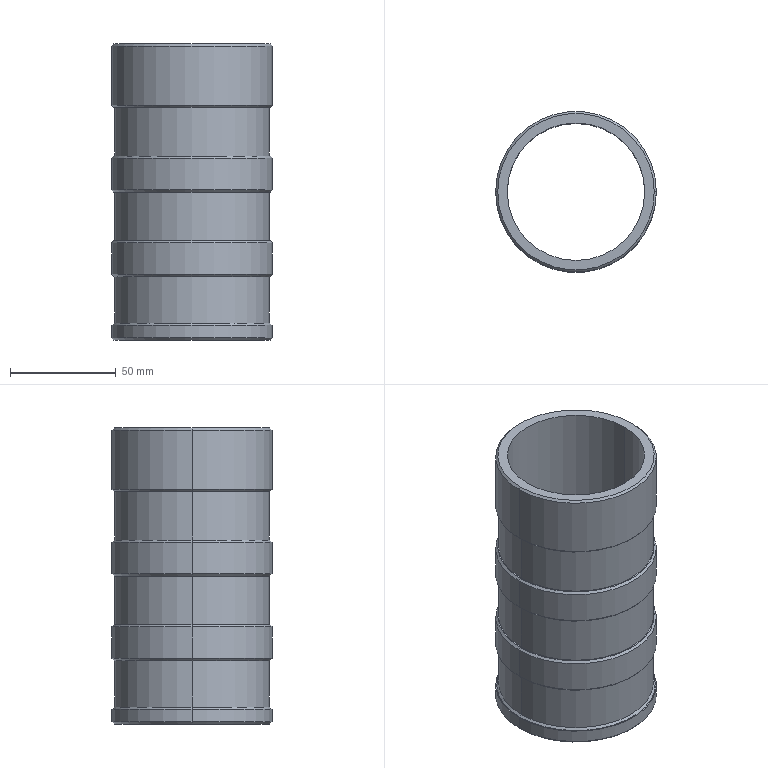Part | SolidWorks | features Chamfer 2, Extrusion 1, ICE 1, LPattern 1 | 1 solid | 40 faces | box 76 x 76 x 140 mm | volume 145605 mm3 | cone 16 | cylinder 16 | plane 8 | commonest cylinder face diameters 76 x8 73 x6 65 x2
STEP:
#1=CARTESIAN_POINT('',(-37.,0.,110.));
#2=VERTEX_POINT('',#1);
#3=CARTESIAN_POINT('',(37.,0.,110.));
#4=VERTEX_POINT('',#3);
#5=CARTESIAN_POINT('',(0.,0.,110.));
#6=DIRECTION('',(0.,0.,-1.));
#7=DIRECTION('',(1.,0.,0.));
#8=AXIS2_PLACEMENT_3D('',#5,#6,#7);
#9=CIRCLE('',#8,37.);
#10=EDGE_CURVE('',#2,#4,#9,.T.);
#11=ORIENTED_EDGE('',*,*,#10,.F.);
#12=CARTESIAN_POINT('',(-38.,0.,111.));
#13=VERTEX_POINT('',#12);
#14=CARTESIAN_POINT('',(-38.,0.,111.));
#15=DIRECTION('',(-0.7071,0.,0.7071));
#16=VECTOR('',#15,1000.);
#17=LINE('',#14,#16);
#18=EDGE_CURVE('',#2,#13,#17,.T.);
#19=ORIENTED_EDGE('',*,*,#18,.T.);
#20=CARTESIAN_POINT('',(38.,0.,111.));
#21=VERTEX_POINT('',#20);
#22=CARTESIAN_POINT('',(0.,0.,111.));
#23=DIRECTION('',(0.,0.,1.));
#24=DIRECTION('',(1.,0.,0.));
#25=AXIS2_PLACEMENT_3D('',#22,#23,#24);
#26=CIRCLE('',#25,38.);
#27=EDGE_CURVE('',#21,#13,#26,.T.);
#28=ORIENTED_EDGE('',*,*,#27,.F.);
#29=CARTESIAN_POINT('',(38.,0.,111.));
#30=DIRECTION('',(0.7071,0.,0.7071));
#31=VECTOR('',#30,1000.);
#32=LINE('',#29,#31);
#33=EDGE_CURVE('',#4,#21,#32,.T.);
#34=ORIENTED_EDGE('',*,*,#33,.F.);
#35=EDGE_LOOP('',(#11,#19,#28,#34));
#36=FACE_OUTER_BOUND('',#35,.T.);
#37=CARTESIAN_POINT('',(0.,0.,111.));
#38=DIRECTION('',(0.,0.,1.));
#39=DIRECTION('',(1.,0.,0.));
#40=AXIS2_PLACEMENT_3D('',#37,#38,#39);
#41=CONICAL_SURFACE('',#40,38.,0.7854);
#42=ADVANCED_FACE('',(#36),#41,.T.);
#43=CARTESIAN_POINT('',(37.,0.,87.));
#44=VERTEX_POINT('',#43);
#45=CARTESIAN_POINT('',(-37.,0.,87.));
#46=VERTEX_POINT('',#45);
#47=CARTESIAN_POINT('',(0.,0.,87.));
#48=DIRECTION('',(0.,0.,1.));
#49=DIRECTION('',(1.,0.,0.));
#50=AXIS2_PLACEMENT_3D('',#47,#48,#49);
#51=CIRCLE('',#50,37.);
#52=EDGE_CURVE('',#44,#46,#51,.T.);
#53=ORIENTED_EDGE('',*,*,#52,.F.);
#54=CARTESIAN_POINT('',(38.,0.,86.));
#55=VERTEX_POINT('',#54);
#56=CARTESIAN_POINT('',(37.,0.,87.));
#57=DIRECTION('',(0.7071,0.,-0.7071));
#58=VECTOR('',#57,1000.);
#59=LINE('',#56,#58);
#60=EDGE_CURVE('',#44,#55,#59,.T.);
#61=ORIENTED_EDGE('',*,*,#60,.T.);
#62=CARTESIAN_POINT('',(-38.,0.,86.));
#63=VERTEX_POINT('',#62);
#64=CARTESIAN_POINT('',(0.,0.,86.));
#65=DIRECTION('',(0.,0.,-1.));
#66=DIRECTION('',(1.,0.,0.));
#67=AXIS2_PLACEMENT_3D('',#64,#65,#66);
#68=CIRCLE('',#67,38.);
#69=EDGE_CURVE('',#63,#55,#68,.T.);
#70=ORIENTED_EDGE('',*,*,#69,.F.);
#71=CARTESIAN_POINT('',(-37.,0.,87.));
#72=DIRECTION('',(-0.7071,0.,-0.7071));
#73=VECTOR('',#72,1000.);
#74=LINE('',#71,#73);
#75=EDGE_CURVE('',#46,#63,#74,.T.);
#76=ORIENTED_EDGE('',*,*,#75,.F.);
#77=EDGE_LOOP('',(#53,#61,#70,#76));
#78=FACE_OUTER_BOUND('',#77,.T.);
#79=CARTESIAN_POINT('',(0.,0.,87.));
#80=DIRECTION('',(0.,0.,-1.));
#81=DIRECTION('',(-1.,0.,0.));
#82=AXIS2_PLACEMENT_3D('',#79,#80,#81);
#83=CONICAL_SURFACE('',#82,37.,0.7854);
#84=ADVANCED_FACE('',(#78),#83,.T.);
#85=CARTESIAN_POINT('',(-37.,0.,70.));
#86=VERTEX_POINT('',#85);
#87=CARTESIAN_POINT('',(37.,0.,70.));
#88=VERTEX_POINT('',#87);
#89=CARTESIAN_POINT('',(0.,0.,70.));
#90=DIRECTION('',(0.,0.,-1.));
#91=DIRECTION('',(1.,0.,0.));
#92=AXIS2_PLACEMENT_3D('',#89,#90,#91);
#93=CIRCLE('',#92,37.);
#94=EDGE_CURVE('',#86,#88,#93,.T.);
#95=ORIENTED_EDGE('',*,*,#94,.F.);
#96=CARTESIAN_POINT('',(-38.,0.,71.));
#97=VERTEX_POINT('',#96);
#98=CARTESIAN_POINT('',(-38.,0.,71.));
#99=DIRECTION('',(-0.7071,0.,0.7071));
#100=VECTOR('',#99,1000.);
#101=LINE('',#98,#100);
#102=EDGE_CURVE('',#86,#97,#101,.T.);
#103=ORIENTED_EDGE('',*,*,#102,.T.);
#104=CARTESIAN_POINT('',(38.,0.,71.));
#105=VERTEX_POINT('',#104);
#106=CARTESIAN_POINT('',(0.,0.,71.));
#107=DIRECTION('',(0.,0.,1.));
#108=DIRECTION('',(1.,0.,0.));
#109=AXIS2_PLACEMENT_3D('',#106,#107,#108);
#110=CIRCLE('',#109,38.);
#111=EDGE_CURVE('',#105,#97,#110,.T.);
#112=ORIENTED_EDGE('',*,*,#111,.F.);
#113=CARTESIAN_POINT('',(38.,0.,71.));
#114=DIRECTION('',(0.7071,0.,0.7071));
#115=VECTOR('',#114,1000.);
#116=LINE('',#113,#115);
#117=EDGE_CURVE('',#88,#105,#116,.T.);
#118=ORIENTED_EDGE('',*,*,#117,.F.);
#119=EDGE_LOOP('',(#95,#103,#112,#118));
#120=FACE_OUTER_BOUND('',#119,.T.);
#121=CARTESIAN_POINT('',(0.,0.,71.));
#122=DIRECTION('',(0.,0.,1.));
#123=DIRECTION('',(1.,0.,0.));
#124=AXIS2_PLACEMENT_3D('',#121,#122,#123);
#125=CONICAL_SURFACE('',#124,38.,0.7854);
#126=ADVANCED_FACE('',(#120),#125,.T.);
#127=CARTESIAN_POINT('',(37.,0.,47.));
#128=VERTEX_POINT('',#127);
#129=CARTESIAN_POINT('',(-37.,0.,47.));
#130=VERTEX_POINT('',#129);
#131=CARTESIAN_POINT('',(0.,0.,47.));
#132=DIRECTION('',(0.,0.,1.));
#133=DIRECTION('',(1.,0.,0.));
#134=AXIS2_PLACEMENT_3D('',#131,#132,#133);
#135=CIRCLE('',#134,37.);
#136=EDGE_CURVE('',#128,#130,#135,.T.);
#137=ORIENTED_EDGE('',*,*,#136,.F.);
#138=CARTESIAN_POINT('',(38.,0.,46.));
#139=VERTEX_POINT('',#138);
#140=CARTESIAN_POINT('',(37.,0.,47.));
#141=DIRECTION('',(0.7071,0.,-0.7071));
#142=VECTOR('',#141,1000.);
#143=LINE('',#140,#142);
#144=EDGE_CURVE('',#128,#139,#143,.T.);
#145=ORIENTED_EDGE('',*,*,#144,.T.);
#146=CARTESIAN_POINT('',(-38.,0.,46.));
#147=VERTEX_POINT('',#146);
#148=CARTESIAN_POINT('',(0.,0.,46.));
#149=DIRECTION('',(0.,0.,-1.));
#150=DIRECTION('',(1.,0.,0.));
#151=AXIS2_PLACEMENT_3D('',#148,#149,#150);
#152=CIRCLE('',#151,38.);
#153=EDGE_CURVE('',#147,#139,#152,.T.);
#154=ORIENTED_EDGE('',*,*,#153,.F.);
#155=CARTESIAN_POINT('',(-37.,0.,47.));
#156=DIRECTION('',(-0.7071,0.,-0.7071));
#157=VECTOR('',#156,1000.);
#158=LINE('',#155,#157);
#159=EDGE_CURVE('',#130,#147,#158,.T.);
#160=ORIENTED_EDGE('',*,*,#159,.F.);
#161=EDGE_LOOP('',(#137,#145,#154,#160));
#162=FACE_OUTER_BOUND('',#161,.T.);
#163=CARTESIAN_POINT('',(0.,0.,47.));
#164=DIRECTION('',(0.,0.,-1.));
#165=DIRECTION('',(-1.,0.,0.));
#166=AXIS2_PLACEMENT_3D('',#163,#164,#165);
#167=CONICAL_SURFACE('',#166,37.,0.7854);
#168=ADVANCED_FACE('',(#162),#167,.T.);
#169=CARTESIAN_POINT('',(-37.,0.,30.));
#170=VERTEX_POINT('',#169);
#171=CARTESIAN_POINT('',(37.,0.,30.));
#172=VERTEX_POINT('',#171);
#173=CARTESIAN_POINT('',(0.,0.,30.));
#174=DIRECTION('',(0.,0.,-1.));
#175=DIRECTION('',(1.,0.,0.));
#176=AXIS2_PLACEMENT_3D('',#173,#174,#175);
#177=CIRCLE('',#176,37.);
#178=EDGE_CURVE('',#170,#172,#177,.T.);
#179=ORIENTED_EDGE('',*,*,#178,.F.);
#180=CARTESIAN_POINT('',(-38.,0.,31.));
#181=VERTEX_POINT('',#180);
#182=CARTESIAN_POINT('',(-38.,0.,31.));
#183=DIRECTION('',(-0.7071,0.,0.7071));
#184=VECTOR('',#183,1000.);
#185=LINE('',#182,#184);
#186=EDGE_CURVE('',#170,#181,#185,.T.);
#187=ORIENTED_EDGE('',*,*,#186,.T.);
#188=CARTESIAN_POINT('',(38.,0.,31.));
#189=VERTEX_POINT('',#188);
#190=CARTESIAN_POINT('',(0.,0.,31.));
#191=DIRECTION('',(0.,0.,1.));
#192=DIRECTION('',(1.,0.,0.));
#193=AXIS2_PLACEMENT_3D('',#190,#191,#192);
#194=CIRCLE('',#193,38.);
#195=EDGE_CURVE('',#189,#181,#194,.T.);
#196=ORIENTED_EDGE('',*,*,#195,.F.);
#197=CARTESIAN_POINT('',(38.,0.,31.));
#198=DIRECTION('',(0.7071,0.,0.7071));
#199=VECTOR('',#198,1000.);
#200=LINE('',#197,#199);
#201=EDGE_CURVE('',#172,#189,#200,.T.);
#202=ORIENTED_EDGE('',*,*,#201,.F.);
#203=EDGE_LOOP('',(#179,#187,#196,#202));
#204=FACE_OUTER_BOUND('',#203,.T.);
#205=CARTESIAN_POINT('',(0.,0.,31.));
#206=DIRECTION('',(0.,0.,1.));
#207=DIRECTION('',(1.,0.,0.));
#208=AXIS2_PLACEMENT_3D('',#205,#206,#207);
#209=CONICAL_SURFACE('',#208,38.,0.7854);
#210=ADVANCED_FACE('',(#204),#209,.T.);
#211=CARTESIAN_POINT('',(36.5,0.,8.));
#212=VERTEX_POINT('',#211);
#213=CARTESIAN_POINT('',(-36.5,0.,8.));
#214=VERTEX_POINT('',#213);
#215=CARTESIAN_POINT('',(0.,0.,8.));
#216=DIRECTION('',(0.,0.,1.));
#217=DIRECTION('',(1.,0.,0.));
#218=AXIS2_PLACEMENT_3D('',#215,#216,#217);
#219=CIRCLE('',#218,36.5);
#220=EDGE_CURVE('',#212,#214,#219,.T.);
#221=ORIENTED_EDGE('',*,*,#220,.F.);
#222=CARTESIAN_POINT('',(37.5,0.,7.));
#223=VERTEX_POINT('',#222);
#224=CARTESIAN_POINT('',(36.5,0.,8.));
#225=DIRECTION('',(0.7071,0.,-0.7071));
#226=VECTOR('',#225,1000.);
#227=LINE('',#224,#226);
#228=EDGE_CURVE('',#212,#223,#227,.T.);
#229=ORIENTED_EDGE('',*,*,#228,.T.);
#230=CARTESIAN_POINT('',(-37.5,0.,7.));
#231=VERTEX_POINT('',#230);
#232=CARTESIAN_POINT('',(0.,0.,7.));
#233=DIRECTION('',(0.,0.,-1.));
#234=DIRECTION('',(1.,0.,0.));
#235=AXIS2_PLACEMENT_3D('',#232,#233,#234);
#236=CIRCLE('',#235,37.5);
#237=EDGE_CURVE('',#231,#223,#236,.T.);
#238=ORIENTED_EDGE('',*,*,#237,.F.);
#239=CARTESIAN_POINT('',(-36.5,0.,8.));
#240=DIRECTION('',(-0.7071,0.,-0.7071));
#241=VECTOR('',#240,1000.);
#242=LINE('',#239,#241);
#243=EDGE_CURVE('',#214,#231,#242,.T.);
#244=ORIENTED_EDGE('',*,*,#243,.F.);
#245=EDGE_LOOP('',(#221,#229,#238,#244));
#246=FACE_OUTER_BOUND('',#245,.T.);
#247=CARTESIAN_POINT('',(0.,0.,8.));
#248=DIRECTION('',(0.,0.,-1.));
#249=DIRECTION('',(-1.,0.,0.));
#250=AXIS2_PLACEMENT_3D('',#247,#248,#249);
#251=CONICAL_SURFACE('',#250,36.5,0.7854);
#252=ADVANCED_FACE('',(#246),#251,.T.);
#253=CARTESIAN_POINT('',(-37.,0.,0.));
#254=VERTEX_POINT('',#253);
#255=CARTESIAN_POINT('',(37.,0.,0.));
#256=VERTEX_POINT('',#255);
#257=CARTESIAN_POINT('',(0.,0.,0.));
#258=DIRECTION('',(0.,0.,-1.));
#259=DIRECTION('',(1.,0.,0.));
#260=AXIS2_PLACEMENT_3D('',#257,#258,#259);
#261=CIRCLE('',#260,37.);
#262=EDGE_CURVE('',#254,#256,#261,.T.);
#263=ORIENTED_EDGE('',*,*,#262,.F.);
#264=CARTESIAN_POINT('',(-38.,0.,1.));
#265=VERTEX_POINT('',#264);
#266=CARTESIAN_POINT('',(-38.,0.,1.));
#267=DIRECTION('',(-0.7071,0.,0.7071));
#268=VECTOR('',#267,1000.);
#269=LINE('',#266,#268);
#270=EDGE_CURVE('',#254,#265,#269,.T.);
#271=ORIENTED_EDGE('',*,*,#270,.T.);
#272=CARTESIAN_POINT('',(38.,0.,1.));
#273=VERTEX_POINT('',#272);
#274=CARTESIAN_POINT('',(0.,0.,1.));
#275=DIRECTION('',(0.,0.,1.));
#276=DIRECTION('',(1.,0.,0.));
#277=AXIS2_PLACEMENT_3D('',#274,#275,#276);
#278=CIRCLE('',#277,38.);
#279=EDGE_CURVE('',#273,#265,#278,.T.);
#280=ORIENTED_EDGE('',*,*,#279,.F.);
#281=CARTESIAN_POINT('',(38.,0.,1.));
#282=DIRECTION('',(0.7071,0.,0.7071));
#283=VECTOR('',#282,1000.);
#284=LINE('',#281,#283);
#285=EDGE_CURVE('',#256,#273,#284,.T.);
#286=ORIENTED_EDGE('',*,*,#285,.F.);
#287=EDGE_LOOP('',(#263,#271,#280,#286));
#288=FACE_OUTER_BOUND('',#287,.T.);
#289=CARTESIAN_POINT('',(0.,0.,1.));
#290=DIRECTION('',(0.,0.,1.));
#291=DIRECTION('',(1.,0.,0.));
#292=AXIS2_PLACEMENT_3D('',#289,#290,#291);
#293=CONICAL_SURFACE('',#292,38.,0.7854);
#294=ADVANCED_FACE('',(#288),#293,.T.);
#295=ORIENTED_EDGE('',*,*,#153,.T.);
#296=CARTESIAN_POINT('',(38.,0.,140.));
#297=DIRECTION('',(0.,0.,-1.));
#298=VECTOR('',#297,1000.);
#299=LINE('',#296,#298);
#300=EDGE_CURVE('',#139,#189,#299,.T.);
#301=ORIENTED_EDGE('',*,*,#300,.T.);
#302=ORIENTED_EDGE('',*,*,#195,.T.);
#303=CARTESIAN_POINT('',(-38.,0.,140.));
#304=DIRECTION('',(0.,0.,-1.));
#305=VECTOR('',#304,1000.);
#306=LINE('',#303,#305);
#307=EDGE_CURVE('',#147,#181,#306,.T.);
#308=ORIENTED_EDGE('',*,*,#307,.F.);
#309=EDGE_LOOP('',(#295,#301,#302,#308));
#310=FACE_OUTER_BOUND('',#309,.T.);
#311=CARTESIAN_POINT('',(0.,0.,140.));
#312=DIRECTION('',(0.,0.,-1.));
#313=DIRECTION('',(-1.,0.,0.));
#314=AXIS2_PLACEMENT_3D('',#311,#312,#313);
#315=CYLINDRICAL_SURFACE('',#314,38.);
#316=ADVANCED_FACE('',(#310),#315,.T.);
#317=CARTESIAN_POINT('',(36.5,0.,47.));
#318=VERTEX_POINT('',#317);
#319=CARTESIAN_POINT('',(-36.5,0.,47.));
#320=VERTEX_POINT('',#319);
#321=CARTESIAN_POINT('',(0.,0.,47.));
#322=DIRECTION('',(0.,0.,1.));
#323=DIRECTION('',(1.,0.,0.));
#324=AXIS2_PLACEMENT_3D('',#321,#322,#323);
#325=CIRCLE('',#324,36.5);
#326=EDGE_CURVE('',#318,#320,#325,.T.);
#327=ORIENTED_EDGE('',*,*,#326,.T.);
#328=CARTESIAN_POINT('',(-36.5,0.,70.));
#329=VERTEX_POINT('',#328);
#330=CARTESIAN_POINT('',(-36.5,0.,47.));
#331=DIRECTION('',(0.,0.,1.));
#332=VECTOR('',#331,1000.);
#333=LINE('',#330,#332);
#334=EDGE_CURVE('',#320,#329,#333,.T.);
#335=ORIENTED_EDGE('',*,*,#334,.T.);
#336=CARTESIAN_POINT('',(36.5,0.,70.));
#337=VERTEX_POINT('',#336);
#338=CARTESIAN_POINT('',(0.,0.,70.));
#339=DIRECTION('',(0.,0.,1.));
#340=DIRECTION('',(1.,0.,0.));
#341=AXIS2_PLACEMENT_3D('',#338,#339,#340);
#342=CIRCLE('',#341,36.5);
#343=EDGE_CURVE('',#337,#329,#342,.T.);
#344=ORIENTED_EDGE('',*,*,#343,.F.);
#345=CARTESIAN_POINT('',(36.5,0.,47.));
#346=DIRECTION('',(0.,0.,1.));
#347=VECTOR('',#346,1000.);
#348=LINE('',#345,#347);
#349=EDGE_CURVE('',#318,#337,#348,.T.);
#350=ORIENTED_EDGE('',*,*,#349,.F.);
#351=EDGE_LOOP('',(#327,#335,#344,#350));
#352=FACE_OUTER_BOUND('',#351,.T.);
#353=CARTESIAN_POINT('',(0.,0.,47.));
#354=DIRECTION('',(0.,0.,1.));
#355=DIRECTION('',(1.,0.,0.));
#356=AXIS2_PLACEMENT_3D('',#353,#354,#355);
#357=CYLINDRICAL_SURFACE('',#356,36.5);
#358=ADVANCED_FACE('',(#352),#357,.T.);
#359=ORIENTED_EDGE('',*,*,#220,.T.);
#360=CARTESIAN_POINT('',(-36.5,0.,30.));
#361=VERTEX_POINT('',#360);
#362=CARTESIAN_POINT('',(-36.5,0.,7.));
#363=DIRECTION('',(0.,0.,1.));
#364=VECTOR('',#363,1000.);
#365=LINE('',#362,#364);
#366=EDGE_CURVE('',#214,#361,#365,.T.);
#367=ORIENTED_EDGE('',*,*,#366,.T.);
#368=CARTESIAN_POINT('',(36.5,0.,30.));
#369=VERTEX_POINT('',#368);
#370=CARTESIAN_POINT('',(0.,0.,30.));
#371=DIRECTION('',(0.,0.,1.));
#372=DIRECTION('',(1.,0.,0.));
#373=AXIS2_PLACEMENT_3D('',#370,#371,#372);
#374=CIRCLE('',#373,36.5);
#375=EDGE_CURVE('',#369,#361,#374,.T.);
#376=ORIENTED_EDGE('',*,*,#375,.F.);
#377=CARTESIAN_POINT('',(36.5,0.,7.));
#378=DIRECTION('',(0.,0.,1.));
#379=VECTOR('',#378,1000.);
#380=LINE('',#377,#379);
#381=EDGE_CURVE('',#212,#369,#380,.T.);
#382=ORIENTED_EDGE('',*,*,#381,.F.);
#383=EDGE_LOOP('',(#359,#367,#376,#382));
#384=FACE_OUTER_BOUND('',#383,.T.);
#385=CARTESIAN_POINT('',(0.,0.,7.));
#386=DIRECTION('',(0.,0.,1.));
#387=DIRECTION('',(1.,0.,0.));
#388=AXIS2_PLACEMENT_3D('',#385,#386,#387);
#389=CYLINDRICAL_SURFACE('',#388,36.5);
#390=ADVANCED_FACE('',(#384),#389,.T.);
#391=CARTESIAN_POINT('',(36.5,0.,87.));
#392=VERTEX_POINT('',#391);
#393=CARTESIAN_POINT('',(-36.5,0.,87.));
#394=VERTEX_POINT('',#393);
#395=CARTESIAN_POINT('',(0.,0.,87.));
#396=DIRECTION('',(0.,0.,1.));
#397=DIRECTION('',(1.,0.,0.));
#398=AXIS2_PLACEMENT_3D('',#395,#396,#397);
#399=CIRCLE('',#398,36.5);
#400=EDGE_CURVE('',#392,#394,#399,.T.);
#401=ORIENTED_EDGE('',*,*,#400,.T.);
#402=CARTESIAN_POINT('',(-36.5,0.,110.));
#403=VERTEX_POINT('',#402);
#404=CARTESIAN_POINT('',(-36.5,0.,87.));
#405=DIRECTION('',(0.,0.,1.));
#406=VECTOR('',#405,1000.);
#407=LINE('',#404,#406);
#408=EDGE_CURVE('',#394,#403,#407,.T.);
#409=ORIENTED_EDGE('',*,*,#408,.T.);
#410=CARTESIAN_POINT('',(36.5,0.,110.));
#411=VERTEX_POINT('',#410);
#412=CARTESIAN_POINT('',(0.,0.,110.));
#413=DIRECTION('',(0.,0.,1.));
#414=DIRECTION('',(1.,0.,0.));
#415=AXIS2_PLACEMENT_3D('',#412,#413,#414);
#416=CIRCLE('',#415,36.5);
#417=EDGE_CURVE('',#411,#403,#416,.T.);
#418=ORIENTED_EDGE('',*,*,#417,.F.);
#419=CARTESIAN_POINT('',(36.5,0.,87.));
#420=DIRECTION('',(0.,0.,1.));
#421=VECTOR('',#420,1000.);
#422=LINE('',#419,#421);
#423=EDGE_CURVE('',#392,#411,#422,.T.);
#424=ORIENTED_EDGE('',*,*,#423,.F.);
#425=EDGE_LOOP('',(#401,#409,#418,#424));
#426=FACE_OUTER_BOUND('',#425,.T.);
#427=CARTESIAN_POINT('',(0.,0.,87.));
#428=DIRECTION('',(0.,0.,1.));
#429=DIRECTION('',(1.,0.,0.));
#430=AXIS2_PLACEMENT_3D('',#427,#428,#429);
#431=CYLINDRICAL_SURFACE('',#430,36.5);
#432=ADVANCED_FACE('',(#426),#431,.T.);
#433=CARTESIAN_POINT('',(37.,0.,140.));
#434=VERTEX_POINT('',#433);
#435=CARTESIAN_POINT('',(-37.,0.,140.));
#436=VERTEX_POINT('',#435);
#437=CARTESIAN_POINT('',(0.,0.,140.));
#438=DIRECTION('',(0.,0.,1.));
#439=DIRECTION('',(1.,0.,0.));
#440=AXIS2_PLACEMENT_3D('',#437,#438,#439);
#441=CIRCLE('',#440,37.);
#442=EDGE_CURVE('',#434,#436,#441,.T.);
#443=ORIENTED_EDGE('',*,*,#442,.F.);
#444=CARTESIAN_POINT('',(38.,0.,139.));
#445=VERTEX_POINT('',#444);
#446=CARTESIAN_POINT('',(37.,0.,140.));
#447=DIRECTION('',(0.7071,0.,-0.7071));
#448=VECTOR('',#447,1000.);
#449=LINE('',#446,#448);
#450=EDGE_CURVE('',#434,#445,#449,.T.);
#451=ORIENTED_EDGE('',*,*,#450,.T.);
#452=CARTESIAN_POINT('',(-38.,0.,139.));
#453=VERTEX_POINT('',#452);
#454=CARTESIAN_POINT('',(0.,0.,139.));
#455=DIRECTION('',(0.,0.,-1.));
#456=DIRECTION('',(1.,0.,0.));
#457=AXIS2_PLACEMENT_3D('',#454,#455,#456);
#458=CIRCLE('',#457,38.);
#459=EDGE_CURVE('',#453,#445,#458,.T.);
#460=ORIENTED_EDGE('',*,*,#459,.F.);
#461=CARTESIAN_POINT('',(-37.,0.,140.));
#462=DIRECTION('',(-0.7071,0.,-0.7071));
#463=VECTOR('',#462,1000.);
#464=LINE('',#461,#463);
#465=EDGE_CURVE('',#436,#453,#464,.T.);
#466=ORIENTED_EDGE('',*,*,#465,.F.);
#467=EDGE_LOOP('',(#443,#451,#460,#466));
#468=FACE_OUTER_BOUND('',#467,.T.);
#469=CARTESIAN_POINT('',(0.,0.,140.));
#470=DIRECTION('',(0.,0.,-1.));
#471=DIRECTION('',(-1.,0.,0.));
#472=AXIS2_PLACEMENT_3D('',#469,#470,#471);
#473=CONICAL_SURFACE('',#472,37.,0.7854);
#474=ADVANCED_FACE('',(#468),#473,.T.);
#475=CARTESIAN_POINT('',(-32.5,0.,140.));
#476=VERTEX_POINT('',#475);
#477=CARTESIAN_POINT('',(32.5,0.,140.));
#478=VERTEX_POINT('',#477);
#479=CARTESIAN_POINT('',(0.,0.,140.));
#480=DIRECTION('',(0.,0.,1.));
#481=DIRECTION('',(1.,0.,0.));
#482=AXIS2_PLACEMENT_3D('',#479,#480,#481);
#483=CIRCLE('',#482,32.5);
#484=EDGE_CURVE('',#476,#478,#483,.T.);
#485=ORIENTED_EDGE('',*,*,#484,.T.);
#486=CARTESIAN_POINT('',(32.5,0.,0.));
#487=VERTEX_POINT('',#486);
#488=CARTESIAN_POINT('',(32.5,0.,140.));
#489=DIRECTION('',(0.,0.,-1.));
#490=VECTOR('',#489,1000.);
#491=LINE('',#488,#490);
#492=EDGE_CURVE('',#478,#487,#491,.T.);
#493=ORIENTED_EDGE('',*,*,#492,.T.);
#494=CARTESIAN_POINT('',(-32.5,0.,0.));
#495=VERTEX_POINT('',#494);
#496=CARTESIAN_POINT('',(0.,0.,0.));
#497=DIRECTION('',(0.,0.,1.));
#498=DIRECTION('',(1.,0.,0.));
#499=AXIS2_PLACEMENT_3D('',#496,#497,#498);
#500=CIRCLE('',#499,32.5);
#501=EDGE_CURVE('',#495,#487,#500,.T.);
#502=ORIENTED_EDGE('',*,*,#501,.F.);
#503=CARTESIAN_POINT('',(-32.5,0.,140.));
#504=DIRECTION('',(0.,0.,-1.));
#505=VECTOR('',#504,1000.);
#506=LINE('',#503,#505);
#507=EDGE_CURVE('',#476,#495,#506,.T.);
#508=ORIENTED_EDGE('',*,*,#507,.F.);
#509=EDGE_LOOP('',(#485,#493,#502,#508));
#510=FACE_OUTER_BOUND('',#509,.T.);
#511=CARTESIAN_POINT('',(0.,0.,140.));
#512=DIRECTION('',(0.,0.,-1.));
#513=DIRECTION('',(-1.,0.,0.));
#514=AXIS2_PLACEMENT_3D('',#511,#512,#513);
#515=CYLINDRICAL_SURFACE('',#514,32.5);
#516=ADVANCED_FACE('',(#510),#515,.F.);
#517=ORIENTED_EDGE('',*,*,#459,.T.);
#518=CARTESIAN_POINT('',(38.,0.,140.));
#519=DIRECTION('',(0.,0.,-1.));
#520=VECTOR('',#519,1000.);
#521=LINE('',#518,#520);
#522=EDGE_CURVE('',#445,#21,#521,.T.);
#523=ORIENTED_EDGE('',*,*,#522,.T.);
#524=ORIENTED_EDGE('',*,*,#27,.T.);
#525=CARTESIAN_POINT('',(-38.,0.,140.));
#526=DIRECTION('',(0.,0.,-1.));
#527=VECTOR('',#526,1000.);
#528=LINE('',#525,#527);
#529=EDGE_CURVE('',#453,#13,#528,.T.);
#530=ORIENTED_EDGE('',*,*,#529,.F.);
#531=EDGE_LOOP('',(#517,#523,#524,#530));
#532=FACE_OUTER_BOUND('',#531,.T.);
#533=CARTESIAN_POINT('',(0.,0.,140.));
#534=DIRECTION('',(0.,0.,-1.));
#535=DIRECTION('',(-1.,0.,0.));
#536=AXIS2_PLACEMENT_3D('',#533,#534,#535);
#537=CYLINDRICAL_SURFACE('',#536,38.);
#538=ADVANCED_FACE('',(#532),#537,.T.);
#539=ORIENTED_EDGE('',*,*,#69,.T.);
#540=CARTESIAN_POINT('',(38.,0.,140.));
#541=DIRECTION('',(0.,0.,-1.));
#542=VECTOR('',#541,1000.);
#543=LINE('',#540,#542);
#544=EDGE_CURVE('',#55,#105,#543,.T.);
#545=ORIENTED_EDGE('',*,*,#544,.T.);
#546=ORIENTED_EDGE('',*,*,#111,.T.);
#547=CARTESIAN_POINT('',(-38.,0.,140.));
#548=DIRECTION('',(0.,0.,-1.));
#549=VECTOR('',#548,1000.);
#550=LINE('',#547,#549);
#551=EDGE_CURVE('',#63,#97,#550,.T.);
#552=ORIENTED_EDGE('',*,*,#551,.F.);
#553=EDGE_LOOP('',(#539,#545,#546,#552));
#554=FACE_OUTER_BOUND('',#553,.T.);
#555=CARTESIAN_POINT('',(0.,0.,140.));
#556=DIRECTION('',(0.,0.,-1.));
#557=DIRECTION('',(-1.,0.,0.));
#558=AXIS2_PLACEMENT_3D('',#555,#556,#557);
#559=CYLINDRICAL_SURFACE('',#558,38.);
#560=ADVANCED_FACE('',(#554),#559,.T.);
#561=CARTESIAN_POINT('',(38.,0.,7.));
#562=VERTEX_POINT('',#561);
#563=CARTESIAN_POINT('',(-38.,0.,7.));
#564=VERTEX_POINT('',#563);
#565=CARTESIAN_POINT('',(0.,0.,7.));
#566=DIRECTION('',(0.,0.,1.));
#567=DIRECTION('',(1.,0.,0.));
#568=AXIS2_PLACEMENT_3D('',#565,#566,#567);
#569=CIRCLE('',#568,38.);
#570=EDGE_CURVE('',#562,#564,#569,.T.);
#571=ORIENTED_EDGE('',*,*,#570,.F.);
#572=CARTESIAN_POINT('',(38.,0.,140.));
#573=DIRECTION('',(0.,0.,-1.));
#574=VECTOR('',#573,1000.);
#575=LINE('',#572,#574);
#576=EDGE_CURVE('',#562,#273,#575,.T.);
#577=ORIENTED_EDGE('',*,*,#576,.T.);
#578=ORIENTED_EDGE('',*,*,#279,.T.);
#579=CARTESIAN_POINT('',(-38.,0.,140.));
#580=DIRECTION('',(0.,0.,-1.));
#581=VECTOR('',#580,1000.);
#582=LINE('',#579,#581);
#583=EDGE_CURVE('',#564,#265,#582,.T.);
#584=ORIENTED_EDGE('',*,*,#583,.F.);
#585=EDGE_LOOP('',(#571,#577,#578,#584));
#586=FACE_OUTER_BOUND('',#585,.T.);
#587=CARTESIAN_POINT('',(0.,0.,140.));
#588=DIRECTION('',(0.,0.,-1.));
#589=DIRECTION('',(-1.,0.,0.));
#590=AXIS2_PLACEMENT_3D('',#587,#588,#589);
#591=CYLINDRICAL_SURFACE('',#590,38.);
#592=ADVANCED_FACE('',(#586),#591,.T.);
#593=ORIENTED_EDGE('',*,*,#576,.F.);
#594=CARTESIAN_POINT('',(0.,0.,7.));
#595=DIRECTION('',(0.,0.,1.));
#596=DIRECTION('',(1.,0.,0.));
#597=AXIS2_PLACEMENT_3D('',#594,#595,#596);
#598=CIRCLE('',#597,38.);
#599=EDGE_CURVE('',#564,#562,#598,.T.);
#600=ORIENTED_EDGE('',*,*,#599,.F.);
#601=ORIENTED_EDGE('',*,*,#583,.T.);
#602=CARTESIAN_POINT('',(0.,0.,1.));
#603=DIRECTION('',(0.,0.,1.));
#604=DIRECTION('',(1.,0.,0.));
#605=AXIS2_PLACEMENT_3D('',#602,#603,#604);
#606=CIRCLE('',#605,38.);
#607=EDGE_CURVE('',#265,#273,#606,.T.);
#608=ORIENTED_EDGE('',*,*,#607,.T.);
#609=EDGE_LOOP('',(#593,#600,#601,#608));
#610=FACE_OUTER_BOUND('',#609,.T.);
#611=CARTESIAN_POINT('',(0.,0.,140.));
#612=DIRECTION('',(0.,0.,-1.));
#613=DIRECTION('',(-1.,0.,0.));
#614=AXIS2_PLACEMENT_3D('',#611,#612,#613);
#615=CYLINDRICAL_SURFACE('',#614,38.);
#616=ADVANCED_FACE('',(#610),#615,.T.);
#617=ORIENTED_EDGE('',*,*,#544,.F.);
#618=CARTESIAN_POINT('',(0.,0.,86.));
#619=DIRECTION('',(0.,0.,-1.));
#620=DIRECTION('',(1.,0.,0.));
#621=AXIS2_PLACEMENT_3D('',#618,#619,#620);
#622=CIRCLE('',#621,38.);
#623=EDGE_CURVE('',#55,#63,#622,.T.);
#624=ORIENTED_EDGE('',*,*,#623,.T.);
#625=ORIENTED_EDGE('',*,*,#551,.T.);
#626=CARTESIAN_POINT('',(0.,0.,71.));
#627=DIRECTION('',(0.,0.,1.));
#628=DIRECTION('',(1.,0.,0.));
#629=AXIS2_PLACEMENT_3D('',#626,#627,#628);
#630=CIRCLE('',#629,38.);
#631=EDGE_CURVE('',#97,#105,#630,.T.);
#632=ORIENTED_EDGE('',*,*,#631,.T.);
#633=EDGE_LOOP('',(#617,#624,#625,#632));
#634=FACE_OUTER_BOUND('',#633,.T.);
#635=CARTESIAN_POINT('',(0.,0.,140.));
#636=DIRECTION('',(0.,0.,-1.));
#637=DIRECTION('',(-1.,0.,0.));
#638=AXIS2_PLACEMENT_3D('',#635,#636,#637);
#639=CYLINDRICAL_SURFACE('',#638,38.);
#640=ADVANCED_FACE('',(#634),#639,.T.);
#641=CARTESIAN_POINT('',(0.,0.,140.));
#642=DIRECTION('',(0.,0.,1.));
#643=DIRECTION('',(1.,0.,0.));
#644=AXIS2_PLACEMENT_3D('',#641,#642,#643);
#645=CIRCLE('',#644,37.);
#646=EDGE_CURVE('',#436,#434,#645,.T.);
#647=ORIENTED_EDGE('',*,*,#646,.T.);
#648=ORIENTED_EDGE('',*,*,#442,.T.);
#649=EDGE_LOOP('',(#647,#648));
#650=FACE_OUTER_BOUND('',#649,.T.);
#651=ORIENTED_EDGE('',*,*,#484,.F.);
#652=CARTESIAN_POINT('',(0.,0.,140.));
#653=DIRECTION('',(0.,0.,1.));
#654=DIRECTION('',(1.,0.,0.));
#655=AXIS2_PLACEMENT_3D('',#652,#653,#654);
#656=CIRCLE('',#655,32.5);
#657=EDGE_CURVE('',#478,#476,#656,.T.);
#658=ORIENTED_EDGE('',*,*,#657,.F.);
#659=EDGE_LOOP('',(#651,#658));
#660=FACE_BOUND('',#659,.T.);
#661=CARTESIAN_POINT('',(0.,0.,140.));
#662=DIRECTION('',(0.,0.,1.));
#663=DIRECTION('',(1.,0.,0.));
#664=AXIS2_PLACEMENT_3D('',#661,#662,#663);
#665=PLANE('',#664);
#666=ADVANCED_FACE('',(#650,#660),#665,.T.);
#667=CARTESIAN_POINT('',(0.,0.,0.));
#668=DIRECTION('',(0.,0.,-1.));
#669=DIRECTION('',(1.,0.,0.));
#670=AXIS2_PLACEMENT_3D('',#667,#668,#669);
#671=CIRCLE('',#670,37.);
#672=EDGE_CURVE('',#256,#254,#671,.T.);
#673=ORIENTED_EDGE('',*,*,#672,.T.);
#674=ORIENTED_EDGE('',*,*,#262,.T.);
#675=EDGE_LOOP('',(#673,#674));
#676=FACE_OUTER_BOUND('',#675,.T.);
#677=ORIENTED_EDGE('',*,*,#501,.T.);
#678=CARTESIAN_POINT('',(0.,0.,0.));
#679=DIRECTION('',(0.,0.,1.));
#680=DIRECTION('',(1.,0.,0.));
#681=AXIS2_PLACEMENT_3D('',#678,#679,#680);
#682=CIRCLE('',#681,32.5);
#683=EDGE_CURVE('',#487,#495,#682,.T.);
#684=ORIENTED_EDGE('',*,*,#683,.T.);
#685=EDGE_LOOP('',(#677,#684));
#686=FACE_BOUND('',#685,.T.);
#687=CARTESIAN_POINT('',(0.,0.,0.));
#688=DIRECTION('',(0.,0.,1.));
#689=DIRECTION('',(1.,0.,0.));
#690=AXIS2_PLACEMENT_3D('',#687,#688,#689);
#691=PLANE('',#690);
#692=ADVANCED_FACE('',(#676,#686),#691,.F.);
#693=ORIENTED_EDGE('',*,*,#522,.F.);
#694=CARTESIAN_POINT('',(0.,0.,139.));
#695=DIRECTION('',(0.,0.,-1.));
#696=DIRECTION('',(1.,0.,0.));
#697=AXIS2_PLACEMENT_3D('',#694,#695,#696);
#698=CIRCLE('',#697,38.);
#699=EDGE_CURVE('',#445,#453,#698,.T.);
#700=ORIENTED_EDGE('',*,*,#699,.T.);
#701=ORIENTED_EDGE('',*,*,#529,.T.);
#702=CARTESIAN_POINT('',(0.,0.,111.));
#703=DIRECTION('',(0.,0.,1.));
#704=DIRECTION('',(1.,0.,0.));
#705=AXIS2_PLACEMENT_3D('',#702,#703,#704);
#706=CIRCLE('',#705,38.);
#707=EDGE_CURVE('',#13,#21,#706,.T.);
#708=ORIENTED_EDGE('',*,*,#707,.T.);
#709=EDGE_LOOP('',(#693,#700,#701,#708));
#710=FACE_OUTER_BOUND('',#709,.T.);
#711=CARTESIAN_POINT('',(0.,0.,140.));
#712=DIRECTION('',(0.,0.,-1.));
#713=DIRECTION('',(-1.,0.,0.));
#714=AXIS2_PLACEMENT_3D('',#711,#712,#713);
#715=CYLINDRICAL_SURFACE('',#714,38.);
#716=ADVANCED_FACE('',(#710),#715,.T.);
#717=ORIENTED_EDGE('',*,*,#492,.F.);
#718=ORIENTED_EDGE('',*,*,#657,.T.);
#719=ORIENTED_EDGE('',*,*,#507,.T.);
#720=ORIENTED_EDGE('',*,*,#683,.F.);
#721=EDGE_LOOP('',(#717,#718,#719,#720));
#722=FACE_OUTER_BOUND('',#721,.T.);
#723=CARTESIAN_POINT('',(0.,0.,140.));
#724=DIRECTION('',(0.,0.,-1.));
#725=DIRECTION('',(-1.,0.,0.));
#726=AXIS2_PLACEMENT_3D('',#723,#724,#725);
#727=CYLINDRICAL_SURFACE('',#726,32.5);
#728=ADVANCED_FACE('',(#722),#727,.F.);
#729=ORIENTED_EDGE('',*,*,#450,.F.);
#730=ORIENTED_EDGE('',*,*,#646,.F.);
#731=ORIENTED_EDGE('',*,*,#465,.T.);
#732=ORIENTED_EDGE('',*,*,#699,.F.);
#733=EDGE_LOOP('',(#729,#730,#731,#732));
#734=FACE_OUTER_BOUND('',#733,.T.);
#735=CARTESIAN_POINT('',(0.,0.,140.));
#736=DIRECTION('',(0.,0.,-1.));
#737=DIRECTION('',(-1.,0.,0.));
#738=AXIS2_PLACEMENT_3D('',#735,#736,#737);
#739=CONICAL_SURFACE('',#738,37.,0.7854);
#740=ADVANCED_FACE('',(#734),#739,.T.);
#741=CARTESIAN_POINT('',(0.,0.,87.));
#742=DIRECTION('',(0.,0.,1.));
#743=DIRECTION('',(1.,0.,0.));
#744=AXIS2_PLACEMENT_3D('',#741,#742,#743);
#745=CIRCLE('',#744,37.);
#746=EDGE_CURVE('',#46,#44,#745,.T.);
#747=ORIENTED_EDGE('',*,*,#746,.T.);
#748=ORIENTED_EDGE('',*,*,#52,.T.);
#749=EDGE_LOOP('',(#747,#748));
#750=FACE_OUTER_BOUND('',#749,.T.);
#751=ORIENTED_EDGE('',*,*,#400,.F.);
#752=CARTESIAN_POINT('',(0.,0.,87.));
#753=DIRECTION('',(0.,0.,1.));
#754=DIRECTION('',(1.,0.,0.));
#755=AXIS2_PLACEMENT_3D('',#752,#753,#754);
#756=CIRCLE('',#755,36.5);
#757=EDGE_CURVE('',#394,#392,#756,.T.);
#758=ORIENTED_EDGE('',*,*,#757,.F.);
#759=EDGE_LOOP('',(#751,#758));
#760=FACE_BOUND('',#759,.T.);
#761=CARTESIAN_POINT('',(0.,0.,87.));
#762=DIRECTION('',(0.,0.,1.));
#763=DIRECTION('',(1.,0.,0.));
#764=AXIS2_PLACEMENT_3D('',#761,#762,#763);
#765=PLANE('',#764);
#766=ADVANCED_FACE('',(#750,#760),#765,.T.);
#767=CARTESIAN_POINT('',(0.,0.,110.));
#768=DIRECTION('',(0.,0.,-1.));
#769=DIRECTION('',(1.,0.,0.));
#770=AXIS2_PLACEMENT_3D('',#767,#768,#769);
#771=CIRCLE('',#770,37.);
#772=EDGE_CURVE('',#4,#2,#771,.T.);
#773=ORIENTED_EDGE('',*,*,#772,.T.);
#774=ORIENTED_EDGE('',*,*,#10,.T.);
#775=EDGE_LOOP('',(#773,#774));
#776=FACE_OUTER_BOUND('',#775,.T.);
#777=ORIENTED_EDGE('',*,*,#417,.T.);
#778=CARTESIAN_POINT('',(0.,0.,110.));
#779=DIRECTION('',(0.,0.,1.));
#780=DIRECTION('',(1.,0.,0.));
#781=AXIS2_PLACEMENT_3D('',#778,#779,#780);
#782=CIRCLE('',#781,36.5);
#783=EDGE_CURVE('',#403,#411,#782,.T.);
#784=ORIENTED_EDGE('',*,*,#783,.T.);
#785=EDGE_LOOP('',(#777,#784));
#786=FACE_BOUND('',#785,.T.);
#787=CARTESIAN_POINT('',(0.,0.,110.));
#788=DIRECTION('',(0.,0.,1.));
#789=DIRECTION('',(1.,0.,0.));
#790=AXIS2_PLACEMENT_3D('',#787,#788,#789);
#791=PLANE('',#790);
#792=ADVANCED_FACE('',(#776,#786),#791,.F.);
#793=ORIENTED_EDGE('',*,*,#408,.F.);
#794=ORIENTED_EDGE('',*,*,#757,.T.);
#795=ORIENTED_EDGE('',*,*,#423,.T.);
#796=ORIENTED_EDGE('',*,*,#783,.F.);
#797=EDGE_LOOP('',(#793,#794,#795,#796));
#798=FACE_OUTER_BOUND('',#797,.T.);
#799=CARTESIAN_POINT('',(0.,0.,87.));
#800=DIRECTION('',(0.,0.,1.));
#801=DIRECTION('',(1.,0.,0.));
#802=AXIS2_PLACEMENT_3D('',#799,#800,#801);
#803=CYLINDRICAL_SURFACE('',#802,36.5);
#804=ADVANCED_FACE('',(#798),#803,.T.);
#805=ORIENTED_EDGE('',*,*,#237,.T.);
#806=CARTESIAN_POINT('',(0.,0.,7.));
#807=DIRECTION('',(0.,0.,-1.));
#808=DIRECTION('',(1.,0.,0.));
#809=AXIS2_PLACEMENT_3D('',#806,#807,#808);
#810=CIRCLE('',#809,37.5);
#811=EDGE_CURVE('',#223,#231,#810,.T.);
#812=ORIENTED_EDGE('',*,*,#811,.T.);
#813=EDGE_LOOP('',(#805,#812));
#814=FACE_BOUND('',#813,.T.);
#815=ORIENTED_EDGE('',*,*,#599,.T.);
#816=ORIENTED_EDGE('',*,*,#570,.T.);
#817=EDGE_LOOP('',(#815,#816));
#818=FACE_OUTER_BOUND('',#817,.T.);
#819=CARTESIAN_POINT('',(0.,0.,7.));
#820=DIRECTION('',(0.,0.,1.));
#821=DIRECTION('',(1.,0.,0.));
#822=AXIS2_PLACEMENT_3D('',#819,#820,#821);
#823=PLANE('',#822);
#824=ADVANCED_FACE('',(#814,#818),#823,.T.);
#825=CARTESIAN_POINT('',(0.,0.,30.));
#826=DIRECTION('',(0.,0.,-1.));
#827=DIRECTION('',(1.,0.,0.));
#828=AXIS2_PLACEMENT_3D('',#825,#826,#827);
#829=CIRCLE('',#828,37.);
#830=EDGE_CURVE('',#172,#170,#829,.T.);
#831=ORIENTED_EDGE('',*,*,#830,.T.);
#832=ORIENTED_EDGE('',*,*,#178,.T.);
#833=EDGE_LOOP('',(#831,#832));
#834=FACE_OUTER_BOUND('',#833,.T.);
#835=ORIENTED_EDGE('',*,*,#375,.T.);
#836=CARTESIAN_POINT('',(0.,0.,30.));
#837=DIRECTION('',(0.,0.,1.));
#838=DIRECTION('',(1.,0.,0.));
#839=AXIS2_PLACEMENT_3D('',#836,#837,#838);
#840=CIRCLE('',#839,36.5);
#841=EDGE_CURVE('',#361,#369,#840,.T.);
#842=ORIENTED_EDGE('',*,*,#841,.T.);
#843=EDGE_LOOP('',(#835,#842));
#844=FACE_BOUND('',#843,.T.);
#845=CARTESIAN_POINT('',(0.,0.,30.));
#846=DIRECTION('',(0.,0.,1.));
#847=DIRECTION('',(1.,0.,0.));
#848=AXIS2_PLACEMENT_3D('',#845,#846,#847);
#849=PLANE('',#848);
#850=ADVANCED_FACE('',(#834,#844),#849,.F.);
#851=ORIENTED_EDGE('',*,*,#366,.F.);
#852=CARTESIAN_POINT('',(0.,0.,8.));
#853=DIRECTION('',(0.,0.,1.));
#854=DIRECTION('',(1.,0.,0.));
#855=AXIS2_PLACEMENT_3D('',#852,#853,#854);
#856=CIRCLE('',#855,36.5);
#857=EDGE_CURVE('',#214,#212,#856,.T.);
#858=ORIENTED_EDGE('',*,*,#857,.T.);
#859=ORIENTED_EDGE('',*,*,#381,.T.);
#860=ORIENTED_EDGE('',*,*,#841,.F.);
#861=EDGE_LOOP('',(#851,#858,#859,#860));
#862=FACE_OUTER_BOUND('',#861,.T.);
#863=CARTESIAN_POINT('',(0.,0.,7.));
#864=DIRECTION('',(0.,0.,1.));
#865=DIRECTION('',(1.,0.,0.));
#866=AXIS2_PLACEMENT_3D('',#863,#864,#865);
#867=CYLINDRICAL_SURFACE('',#866,36.5);
#868=ADVANCED_FACE('',(#862),#867,.T.);
#869=CARTESIAN_POINT('',(0.,0.,47.));
#870=DIRECTION('',(0.,0.,1.));
#871=DIRECTION('',(1.,0.,0.));
#872=AXIS2_PLACEMENT_3D('',#869,#870,#871);
#873=CIRCLE('',#872,37.);
#874=EDGE_CURVE('',#130,#128,#873,.T.);
#875=ORIENTED_EDGE('',*,*,#874,.T.);
#876=ORIENTED_EDGE('',*,*,#136,.T.);
#877=EDGE_LOOP('',(#875,#876));
#878=FACE_OUTER_BOUND('',#877,.T.);
#879=ORIENTED_EDGE('',*,*,#326,.F.);
#880=CARTESIAN_POINT('',(0.,0.,47.));
#881=DIRECTION('',(0.,0.,1.));
#882=DIRECTION('',(1.,0.,0.));
#883=AXIS2_PLACEMENT_3D('',#880,#881,#882);
#884=CIRCLE('',#883,36.5);
#885=EDGE_CURVE('',#320,#318,#884,.T.);
#886=ORIENTED_EDGE('',*,*,#885,.F.);
#887=EDGE_LOOP('',(#879,#886));
#888=FACE_BOUND('',#887,.T.);
#889=CARTESIAN_POINT('',(0.,0.,47.));
#890=DIRECTION('',(0.,0.,1.));
#891=DIRECTION('',(1.,0.,0.));
#892=AXIS2_PLACEMENT_3D('',#889,#890,#891);
#893=PLANE('',#892);
#894=ADVANCED_FACE('',(#878,#888),#893,.T.);
#895=CARTESIAN_POINT('',(0.,0.,70.));
#896=DIRECTION('',(0.,0.,-1.));
#897=DIRECTION('',(1.,0.,0.));
#898=AXIS2_PLACEMENT_3D('',#895,#896,#897);
#899=CIRCLE('',#898,37.);
#900=EDGE_CURVE('',#88,#86,#899,.T.);
#901=ORIENTED_EDGE('',*,*,#900,.T.);
#902=ORIENTED_EDGE('',*,*,#94,.T.);
#903=EDGE_LOOP('',(#901,#902));
#904=FACE_OUTER_BOUND('',#903,.T.);
#905=ORIENTED_EDGE('',*,*,#343,.T.);
#906=CARTESIAN_POINT('',(0.,0.,70.));
#907=DIRECTION('',(0.,0.,1.));
#908=DIRECTION('',(1.,0.,0.));
#909=AXIS2_PLACEMENT_3D('',#906,#907,#908);
#910=CIRCLE('',#909,36.5);
#911=EDGE_CURVE('',#329,#337,#910,.T.);
#912=ORIENTED_EDGE('',*,*,#911,.T.);
#913=EDGE_LOOP('',(#905,#912));
#914=FACE_BOUND('',#913,.T.);
#915=CARTESIAN_POINT('',(0.,0.,70.));
#916=DIRECTION('',(0.,0.,1.));
#917=DIRECTION('',(1.,0.,0.));
#918=AXIS2_PLACEMENT_3D('',#915,#916,#917);
#919=PLANE('',#918);
#920=ADVANCED_FACE('',(#904,#914),#919,.F.);
#921=ORIENTED_EDGE('',*,*,#334,.F.);
#922=ORIENTED_EDGE('',*,*,#885,.T.);
#923=ORIENTED_EDGE('',*,*,#349,.T.);
#924=ORIENTED_EDGE('',*,*,#911,.F.);
#925=EDGE_LOOP('',(#921,#922,#923,#924));
#926=FACE_OUTER_BOUND('',#925,.T.);
#927=CARTESIAN_POINT('',(0.,0.,47.));
#928=DIRECTION('',(0.,0.,1.));
#929=DIRECTION('',(1.,0.,0.));
#930=AXIS2_PLACEMENT_3D('',#927,#928,#929);
#931=CYLINDRICAL_SURFACE('',#930,36.5);
#932=ADVANCED_FACE('',(#926),#931,.T.);
#933=ORIENTED_EDGE('',*,*,#300,.F.);
#934=CARTESIAN_POINT('',(0.,0.,46.));
#935=DIRECTION('',(0.,0.,-1.));
#936=DIRECTION('',(1.,0.,0.));
#937=AXIS2_PLACEMENT_3D('',#934,#935,#936);
#938=CIRCLE('',#937,38.);
#939=EDGE_CURVE('',#139,#147,#938,.T.);
#940=ORIENTED_EDGE('',*,*,#939,.T.);
#941=ORIENTED_EDGE('',*,*,#307,.T.);
#942=CARTESIAN_POINT('',(0.,0.,31.));
#943=DIRECTION('',(0.,0.,1.));
#944=DIRECTION('',(1.,0.,0.));
#945=AXIS2_PLACEMENT_3D('',#942,#943,#944);
#946=CIRCLE('',#945,38.);
#947=EDGE_CURVE('',#181,#189,#946,.T.);
#948=ORIENTED_EDGE('',*,*,#947,.T.);
#949=EDGE_LOOP('',(#933,#940,#941,#948));
#950=FACE_OUTER_BOUND('',#949,.T.);
#951=CARTESIAN_POINT('',(0.,0.,140.));
#952=DIRECTION('',(0.,0.,-1.));
#953=DIRECTION('',(-1.,0.,0.));
#954=AXIS2_PLACEMENT_3D('',#951,#952,#953);
#955=CYLINDRICAL_SURFACE('',#954,38.);
#956=ADVANCED_FACE('',(#950),#955,.T.);
#957=ORIENTED_EDGE('',*,*,#270,.F.);
#958=ORIENTED_EDGE('',*,*,#672,.F.);
#959=ORIENTED_EDGE('',*,*,#285,.T.);
#960=ORIENTED_EDGE('',*,*,#607,.F.);
#961=EDGE_LOOP('',(#957,#958,#959,#960));
#962=FACE_OUTER_BOUND('',#961,.T.);
#963=CARTESIAN_POINT('',(0.,0.,1.));
#964=DIRECTION('',(0.,0.,1.));
#965=DIRECTION('',(1.,0.,0.));
#966=AXIS2_PLACEMENT_3D('',#963,#964,#965);
#967=CONICAL_SURFACE('',#966,38.,0.7854);
#968=ADVANCED_FACE('',(#962),#967,.T.);
#969=ORIENTED_EDGE('',*,*,#228,.F.);
#970=ORIENTED_EDGE('',*,*,#857,.F.);
#971=ORIENTED_EDGE('',*,*,#243,.T.);
#972=ORIENTED_EDGE('',*,*,#811,.F.);
#973=EDGE_LOOP('',(#969,#970,#971,#972));
#974=FACE_OUTER_BOUND('',#973,.T.);
#975=CARTESIAN_POINT('',(0.,0.,8.));
#976=DIRECTION('',(0.,0.,-1.));
#977=DIRECTION('',(-1.,0.,0.));
#978=AXIS2_PLACEMENT_3D('',#975,#976,#977);
#979=CONICAL_SURFACE('',#978,36.5,0.7854);
#980=ADVANCED_FACE('',(#974),#979,.T.);
#981=ORIENTED_EDGE('',*,*,#186,.F.);
#982=ORIENTED_EDGE('',*,*,#830,.F.);
#983=ORIENTED_EDGE('',*,*,#201,.T.);
#984=ORIENTED_EDGE('',*,*,#947,.F.);
#985=EDGE_LOOP('',(#981,#982,#983,#984));
#986=FACE_OUTER_BOUND('',#985,.T.);
#987=CARTESIAN_POINT('',(0.,0.,31.));
#988=DIRECTION('',(0.,0.,1.));
#989=DIRECTION('',(1.,0.,0.));
#990=AXIS2_PLACEMENT_3D('',#987,#988,#989);
#991=CONICAL_SURFACE('',#990,38.,0.7854);
#992=ADVANCED_FACE('',(#986),#991,.T.);
#993=ORIENTED_EDGE('',*,*,#144,.F.);
#994=ORIENTED_EDGE('',*,*,#874,.F.);
#995=ORIENTED_EDGE('',*,*,#159,.T.);
#996=ORIENTED_EDGE('',*,*,#939,.F.);
#997=EDGE_LOOP('',(#993,#994,#995,#996));
#998=FACE_OUTER_BOUND('',#997,.T.);
#999=CARTESIAN_POINT('',(0.,0.,47.));
#1000=DIRECTION('',(0.,0.,-1.));
#1001=DIRECTION('',(-1.,0.,0.));
#1002=AXIS2_PLACEMENT_3D('',#999,#1000,#1001);
#1003=CONICAL_SURFACE('',#1002,37.,0.7854);
#1004=ADVANCED_FACE('',(#998),#1003,.T.);
#1005=ORIENTED_EDGE('',*,*,#102,.F.);
#1006=ORIENTED_EDGE('',*,*,#900,.F.);
#1007=ORIENTED_EDGE('',*,*,#117,.T.);
#1008=ORIENTED_EDGE('',*,*,#631,.F.);
#1009=EDGE_LOOP('',(#1005,#1006,#1007,#1008));
#1010=FACE_OUTER_BOUND('',#1009,.T.);
#1011=CARTESIAN_POINT('',(0.,0.,71.));
#1012=DIRECTION('',(0.,0.,1.));
#1013=DIRECTION('',(1.,0.,0.));
#1014=AXIS2_PLACEMENT_3D('',#1011,#1012,#1013);
#1015=CONICAL_SURFACE('',#1014,38.,0.7854);
#1016=ADVANCED_FACE('',(#1010),#1015,.T.);
#1017=ORIENTED_EDGE('',*,*,#60,.F.);
#1018=ORIENTED_EDGE('',*,*,#746,.F.);
#1019=ORIENTED_EDGE('',*,*,#75,.T.);
#1020=ORIENTED_EDGE('',*,*,#623,.F.);
#1021=EDGE_LOOP('',(#1017,#1018,#1019,#1020));
#1022=FACE_OUTER_BOUND('',#1021,.T.);
#1023=CARTESIAN_POINT('',(0.,0.,87.));
#1024=DIRECTION('',(0.,0.,-1.));
#1025=DIRECTION('',(-1.,0.,0.));
#1026=AXIS2_PLACEMENT_3D('',#1023,#1024,#1025);
#1027=CONICAL_SURFACE('',#1026,37.,0.7854);
#1028=ADVANCED_FACE('',(#1022),#1027,.T.);
#1029=ORIENTED_EDGE('',*,*,#18,.F.);
#1030=ORIENTED_EDGE('',*,*,#772,.F.);
#1031=ORIENTED_EDGE('',*,*,#33,.T.);
#1032=ORIENTED_EDGE('',*,*,#707,.F.);
#1033=EDGE_LOOP('',(#1029,#1030,#1031,#1032));
#1034=FACE_OUTER_BOUND('',#1033,.T.);
#1035=CARTESIAN_POINT('',(0.,0.,111.));
#1036=DIRECTION('',(0.,0.,1.));
#1037=DIRECTION('',(1.,0.,0.));
#1038=AXIS2_PLACEMENT_3D('',#1035,#1036,#1037);
#1039=CONICAL_SURFACE('',#1038,38.,0.7854);
#1040=ADVANCED_FACE('',(#1034),#1039,.T.);
#1041=CLOSED_SHELL('',(#42,#84,#126,#168,#210,#252,#294,#316,#358,#390,#432,#474,#516,#538,#560,#592,#616,#640,#666,#692,#716,#728,#740,#766,#792,#804,#824,#850,#868,#894,#920,#932,#956,#968,#980,#992,#1004,#1016,#1028,#1040));
#1042=MANIFOLD_SOLID_BREP('',#1041);
#1043=CARTESIAN_POINT('',(0.,0.,0.));
#1044=DIRECTION('',(0.,0.,1.));
#1045=DIRECTION('',(1.,0.,0.));
#1046=AXIS2_PLACEMENT_3D('',#1043,#1044,#1045);
#1047=(LENGTH_UNIT()NAMED_UNIT(*)SI_UNIT(.MILLI.,.METRE.));
#1048=UNCERTAINTY_MEASURE_WITH_UNIT(LENGTH_MEASURE(0.00001),#1047,'','');
#1049=(NAMED_UNIT(*)PLANE_ANGLE_UNIT()SI_UNIT($,.RADIAN.));
#1050=(NAMED_UNIT(*)SI_UNIT($,.STERADIAN.)SOLID_ANGLE_UNIT());
#1051=(GEOMETRIC_REPRESENTATION_CONTEXT(3)GLOBAL_UNCERTAINTY_ASSIGNED_CONTEXT((#1048))GLOBAL_UNIT_ASSIGNED_CONTEXT((#1047,#1049,#1050))REPRESENTATION_CONTEXT('',''));
#1052=ADVANCED_BREP_SHAPE_REPRESENTATION('',(#1042,#1046),#1051);